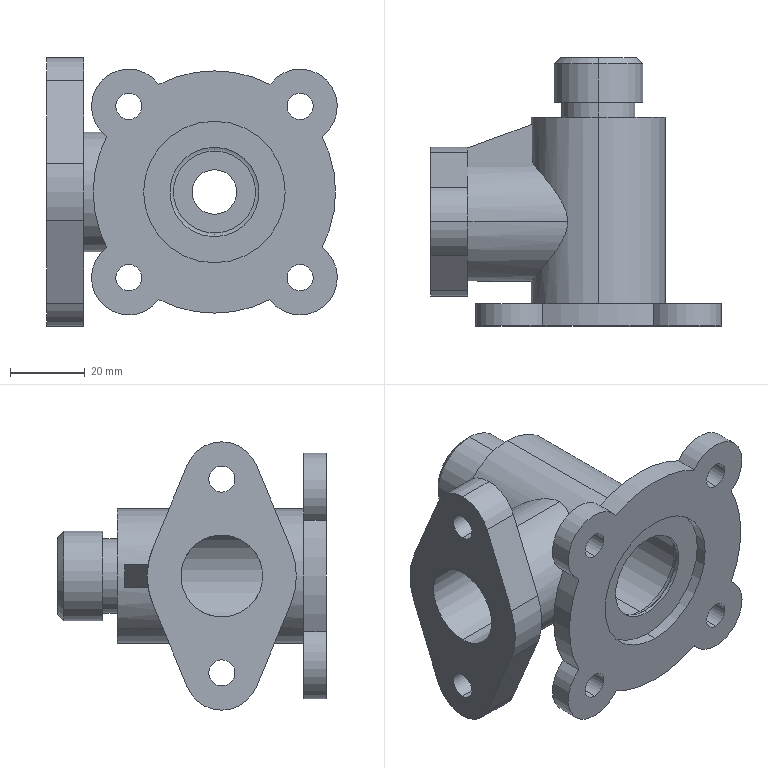Part | SolidWorks | features ICE 13, Chamfer 2, Extrusion 1, Fillet 1, Rib 1, StudWizard 1 | 1 solid | 77 faces | box 77.981 x 72 x 72 mm | volume 74377 mm3 | cylinder 49 | plane 18 | cone 6 | torus 4 | commonest cylinder face diameters 7 x12 20 x11 65 x5 24 x4 32 x3 12 x2